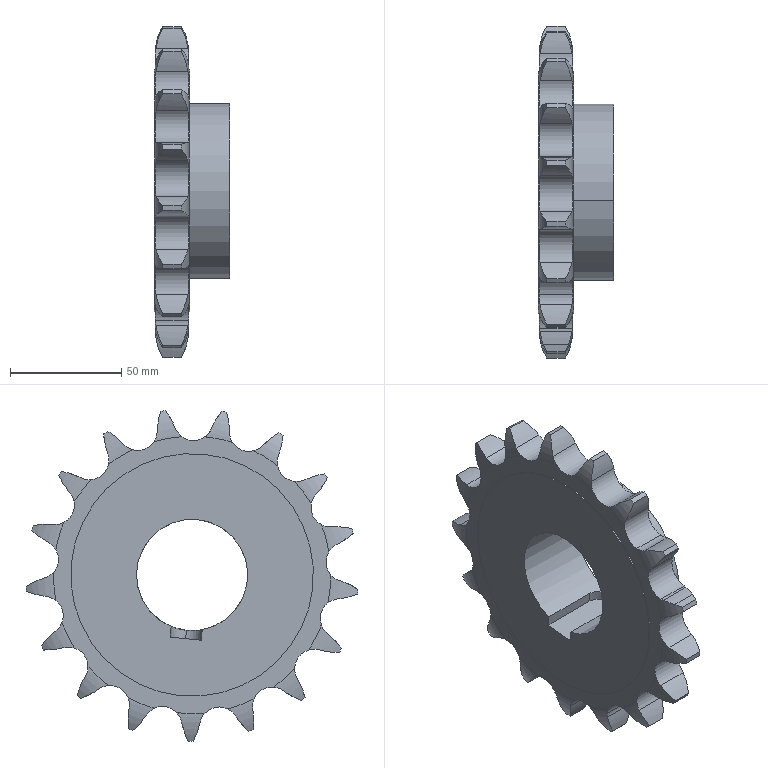Part | STEP file | Cut-Extrude 8 | 1 solid | 137 faces | box 34 x 149.139 x 148.625 mm | volume 228530 mm3 | cylinder 91 | torus 38 | plane 8 | commonest cylinder face diameters 72.413 x39 17.468 x25 149.594 x17 109 x4 14 x2 50 x2